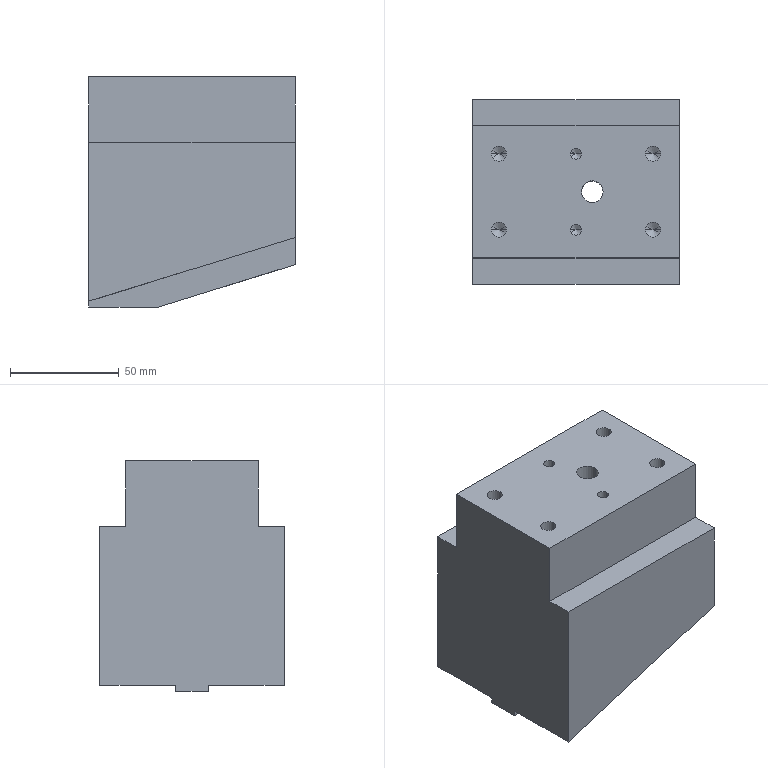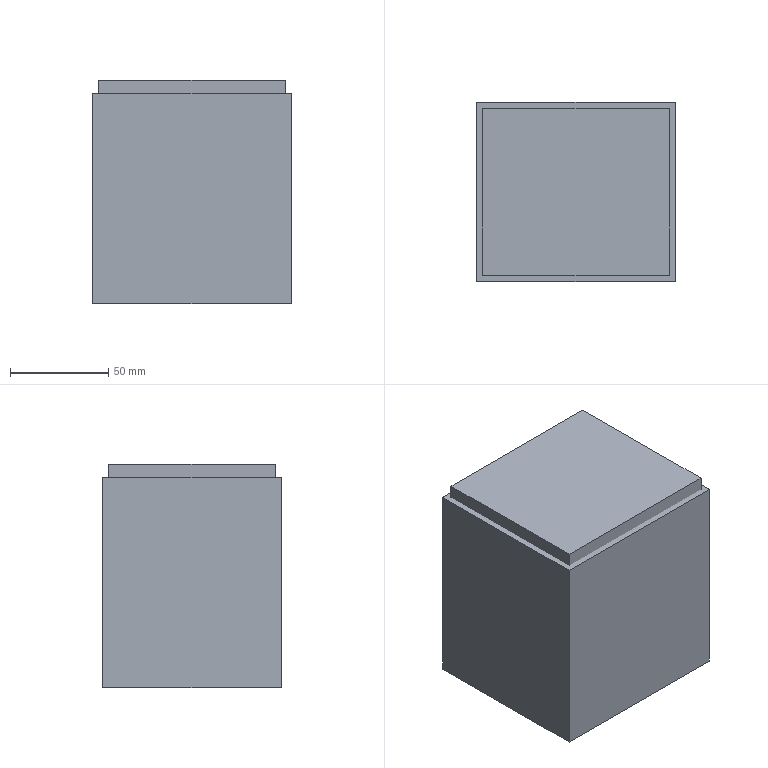CAM job | NX | 3-axis milling, drilling | part box 95 x 85 x 106 mm | stock box 101 x 91 x 114 mm
Tools:
number,name,description,diameter,corner_radius,flute_length,length,flutes
1,D63,Milling Tool-5 Parameters,63.0,0.0,50.0,75.0,2
7,D6A45,Milling Tool-5 Parameters,6.0,0.0,3.0,3.0,2
14,4.8ZT,Drilling Tool,4.8,0.0,35.0,50.0,2
15,5.0JD,Milling Tool-5 Parameters,5.0,0.0,30.0,30.0,4
17,7.0ZT,Drilling Tool,7.0,0.0,35.0,50.0,2
18,8.5ZT,Drilling Tool,8.5,0.0,35.0,50.0,2
10,D10,Milling Tool-5 Parameters,10.0,0.0,50.0,75.0,2
11,D10JING,Milling Tool-5 Parameters,10.0,0.0,50.0,75.0,2
5,D6R0.5,Milling Tool-5 Parameters,6.0,0.5,50.0,75.0,2
Operations:
program,operation,operation_type,tool,method,geometry_group,spindle_rpm,surface_speed,feed_per_tooth,feed_cut,feed_plunge,cut_length_mm,path_length_mm,cut_time_min,machine_time_min
1-115-90-100毛胚,FLOOR_WALL,VolumeBased25DMillingOperation,D63,METHOD,A,6500.0,1286.0,0.0962,1250.0,100.0,569.797,623.797,0.4558,0.4612
1-115-90-100毛胚,DRILLING_COPY_1,Operation,D6A45,METHOD,A,5000.0,94.0,0.025,250.0,0.0,28.0,314.058,0.112,0.1406
1-115-90-100毛胚,DRILLING_COPY_COPY_1,Operation,4.8ZT,METHOD,A,2000.0,15.0,0.03,120.0,0.0,28.884,155.897,0.2407,0.2534
1-115-90-100毛胚,DRILLING_COPY_COPY_1_COPY,Operation,5.0JD,METHOD,A,1000.0,15.0,0.0125,50.0,0.0,26.0,150.128,0.52,0.5324
1-115-90-100毛胚,DRILLING_COPY_COPY_1_COPY_1,Operation,7.0ZT,METHOD,A,2000.0,15.0,0.03,120.0,0.0,80.412,451.166,0.6701,0.7072
1-115-90-100毛胚,DRILLING_COPY_COPY_1_COPY_1_COPY,Operation,8.5ZT,METHOD,A,1200.0,32.0,0.05,120.0,0.0,107.454,274.908,0.8955,0.9122
1-115-90-100毛胚,ZLEVEL_PROFILE_COPY_COPY_1_COPY_COPY_COPY,ZLevelMilling,D10,METHOD,A,9500.0,298.0,0.1579,3000.0,1000.0,11868.139,11955.139,3.988,3.997
1-115-90-100毛胚,ZLEVEL_PROFILE_COPY_COPY_1_COPY_COPY_COPY_1,ZLevelMilling,D10,METHOD,A,9500.0,298.0,0.1579,3000.0,1000.0,11351.511,11438.411,3.816,3.824
1-115-90-100毛胚,ZLEVEL_PROFILE_COPY_COPY_1_COPY_COPY,ZLevelMilling,D10,METHOD,A,9500.0,298.0,0.1579,3000.0,1000.0,21117.309,21417.125,7.102,7.132
1-115-90-100毛胚,ZLEVEL_PROFILE_COPY_COPY_1_COPY_COPY_1,ZLevelMilling,D10JING,METHOD,A,9500.0,298.0,0.0632,1200.0,100.0,1501.746,2018.191,1.252,1.303
1-115-90-100毛胚,ZLEVEL_PROFILE_COPY_COPY_1_COPY_COPY_1_COPY,ZLevelMilling,D10JING,METHOD,A,9500.0,298.0,0.0632,1200.0,100.0,226.755,536.733,0.189,0.22
1-115-90-100毛胚,ZLEVEL_PROFILE_1_COPY_1_COPY_COPY,ZLevelMilling,D6A45,METHOD,A,9500.0,179.0,0.0526,1000.0,100.0,468.928,1307.299,0.4689,0.5528
1-115-90-100毛胚,ZLEVEL_PROFILE_1_COPY_1_COPY_COPY_COPY,ZLevelMilling,D6A45,METHOD,A,9500.0,179.0,0.0526,1000.0,100.0,241.925,550.094,0.2419,0.2727
2-115-90-100毛胚,FLOOR_WALL_COPY,VolumeBased25DMillingOperation,D63,METHOD,B,6500.0,1286.0,0.0962,1250.0,100.0,4366.376,6028.308,3.493,3.659
2-115-90-100毛胚,ZLEVEL_PROFILE_COPY_COPY_1_COPY_COPY_COPY_COPY,ZLevelMilling,D10,METHOD,B,9500.0,298.0,0.1579,3000.0,1000.0,22061.516,22174.516,7.386,7.397
2-115-90-100毛胚,FIXED_CONTOUR_COPY_COPY_COPY,SurfaceContour,D10,METHOD,B,9500.0,89.0,0.1053,2000.0,1000.0,3991.978,4080.914,1.999,2.008
2-115-90-100毛胚,FIXED_CONTOUR_COPY_COPY_COPY_COPY_2,SurfaceContour,D10,METHOD,B,9500.0,89.0,0.1053,2000.0,1000.0,3980.057,4074.057,1.993,2.002
2-115-90-100毛胚,FIXED_CONTOUR_COPY,SurfaceContour,D10,METHOD,B,9500.0,89.0,0.1053,2000.0,1000.0,2439.601,2513.601,1.223,1.23
2-115-90-100毛胚,FIXED_CONTOUR_COPY_COPY_COPY_COPY_1,SurfaceContour,D6R0.5,METHOD,B,9500.0,179.0,0.1579,3000.0,1000.0,37597.957,37686.208,12.549,12.557
2-115-90-100毛胚,FIXED_CONTOUR_COPY_COPY_COPY_COPY_1_COPY,SurfaceContour,D6R0.5,METHOD,B,9500.0,179.0,0.1579,3000.0,1000.0,37474.107,37570.191,12.494,12.503
2-115-90-100毛胚,FIXED_CONTOUR_COPY_COPY_COPY_COPY_1_COPY_COPY,SurfaceContour,D6R0.5,METHOD,B,9500.0,179.0,0.1579,3000.0,1000.0,18640.674,18719.197,6.219,6.227
2-115-90-100毛胚,ZLEVEL_PROFILE_COPY_COPY_1_COPY_COPY_1_COPY_1,ZLevelMilling,D10JING,METHOD,B,9500.0,298.0,0.0632,1200.0,100.0,1198.31,1587.697,0.9986,1.038
2-115-90-100毛胚,FIXED_CONTOUR_COPY_COPY_COPY_COPY,SurfaceContour,D10JING,METHOD,MCS_MILL_B,9000.0,282.0,0.0556,1000.0,1000.0,140.38,220.745,0.1404,0.1484
2-115-90-100毛胚,FIXED_CONTOUR_COPY_COPY_COPY_COPY_COPY,SurfaceContour,D10JING,METHOD,MCS_MILL_B,9000.0,282.0,0.0556,1000.0,1000.0,140.38,220.745,0.1404,0.1484
2-115-90-100毛胚,ZLEVEL_PROFILE_COPY_1_COPY_1_COPY_1_1_COPY_COPY,ZLevelMilling,D10JING,METHOD,B,9000.0,282.0,0.1111,2000.0,800.0,7207.642,7493.599,3.61,3.639
2-115-90-100毛胚,ZLEVEL_PROFILE_COPY_1_COPY_1_COPY_1_1_COPY,ZLevelMilling,D10JING,METHOD,B,9000.0,282.0,0.1111,2000.0,800.0,8302.303,8588.539,4.159,4.187
2-115-90-100毛胚,ZLEVEL_PROFILE_COPY_COPY_1_COPY_COPY_1_COPY_1_COPY_COPY,ZLevelMilling,D10JING,METHOD,B,9500.0,298.0,0.0632,1200.0,100.0,240.533,580.308,0.2004,0.2344
2-115-90-100毛胚,ZLEVEL_PROFILE_COPY_COPY_1_COPY_COPY_1_COPY_1_COPY,ZLevelMilling,D10JING,METHOD,B,9500.0,298.0,0.0632,1200.0,100.0,557.648,1164.756,0.4647,0.5254
2-115-90-100毛胚,FIXED_CONTOUR_COPY_COPY_COPY_COPY_1_COPY_1,SurfaceContour,D6R0.5,METHOD,B,9500.0,179.0,0.1579,3000.0,1000.0,13382.578,13837.66,4.492,4.537